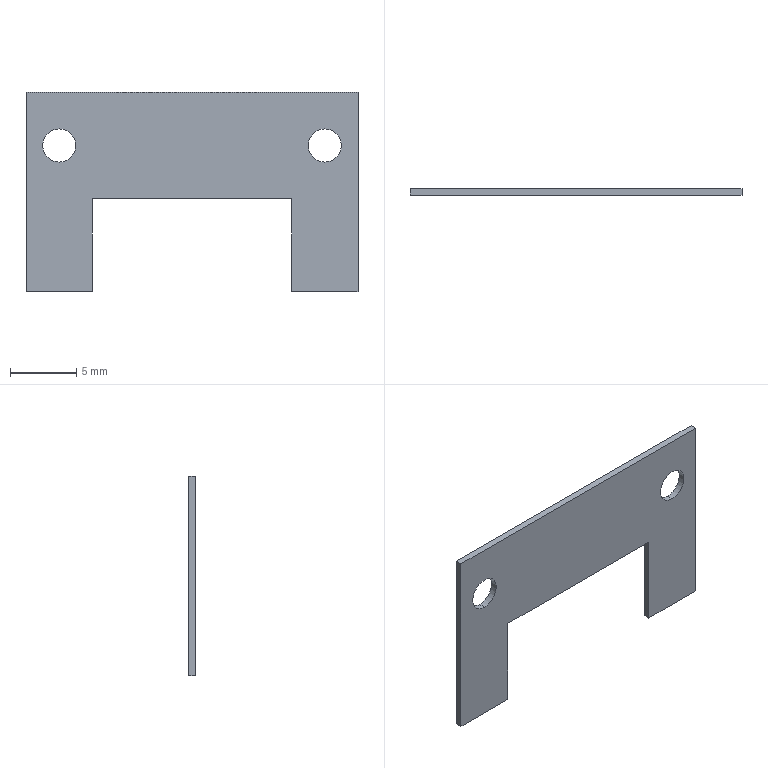Part | SolidWorks | features Extrusion 1 | 1 solid | 14 faces | box 25 x 0.5 x 15 mm | volume 130.091 mm3 | plane 10 | cylinder 4 | commonest cylinder face diameters 2.5 x4
STEP:
#1=CARTESIAN_POINT('',(-10.,0.5,-5.25));
#2=VERTEX_POINT('',#1);
#3=CARTESIAN_POINT('',(-10.,0.5,-2.75));
#4=VERTEX_POINT('',#3);
#5=CARTESIAN_POINT('',(-10.,0.5,-4.));
#6=DIRECTION('',(0.,1.,0.));
#7=DIRECTION('',(0.,0.,1.));
#8=AXIS2_PLACEMENT_3D('',#5,#6,#7);
#9=CIRCLE('',#8,1.25);
#10=EDGE_CURVE('',#2,#4,#9,.T.);
#11=ORIENTED_EDGE('',*,*,#10,.T.);
#12=CARTESIAN_POINT('',(-10.,0.,-2.75));
#13=VERTEX_POINT('',#12);
#14=CARTESIAN_POINT('',(-10.,0.5,-2.75));
#15=DIRECTION('',(0.,-1.,0.));
#16=VECTOR('',#15,1000.);
#17=LINE('',#14,#16);
#18=EDGE_CURVE('',#4,#13,#17,.T.);
#19=ORIENTED_EDGE('',*,*,#18,.T.);
#20=CARTESIAN_POINT('',(-10.,0.,-5.25));
#21=VERTEX_POINT('',#20);
#22=CARTESIAN_POINT('',(-10.,0.,-4.));
#23=DIRECTION('',(0.,1.,0.));
#24=DIRECTION('',(0.,0.,1.));
#25=AXIS2_PLACEMENT_3D('',#22,#23,#24);
#26=CIRCLE('',#25,1.25);
#27=EDGE_CURVE('',#21,#13,#26,.T.);
#28=ORIENTED_EDGE('',*,*,#27,.F.);
#29=CARTESIAN_POINT('',(-10.,0.5,-5.25));
#30=DIRECTION('',(0.,-1.,0.));
#31=VECTOR('',#30,1000.);
#32=LINE('',#29,#31);
#33=EDGE_CURVE('',#2,#21,#32,.T.);
#34=ORIENTED_EDGE('',*,*,#33,.F.);
#35=EDGE_LOOP('',(#11,#19,#28,#34));
#36=FACE_OUTER_BOUND('',#35,.T.);
#37=CARTESIAN_POINT('',(-10.,0.5,-4.));
#38=DIRECTION('',(0.,-1.,0.));
#39=DIRECTION('',(0.,0.,-1.));
#40=AXIS2_PLACEMENT_3D('',#37,#38,#39);
#41=CYLINDRICAL_SURFACE('',#40,1.25);
#42=ADVANCED_FACE('',(#36),#41,.F.);
#43=CARTESIAN_POINT('',(10.,0.5,-5.25));
#44=VERTEX_POINT('',#43);
#45=CARTESIAN_POINT('',(10.,0.5,-2.75));
#46=VERTEX_POINT('',#45);
#47=CARTESIAN_POINT('',(10.,0.5,-4.));
#48=DIRECTION('',(0.,1.,0.));
#49=DIRECTION('',(0.,0.,1.));
#50=AXIS2_PLACEMENT_3D('',#47,#48,#49);
#51=CIRCLE('',#50,1.25);
#52=EDGE_CURVE('',#44,#46,#51,.T.);
#53=ORIENTED_EDGE('',*,*,#52,.T.);
#54=CARTESIAN_POINT('',(10.,0.,-2.75));
#55=VERTEX_POINT('',#54);
#56=CARTESIAN_POINT('',(10.,0.5,-2.75));
#57=DIRECTION('',(0.,-1.,0.));
#58=VECTOR('',#57,1000.);
#59=LINE('',#56,#58);
#60=EDGE_CURVE('',#46,#55,#59,.T.);
#61=ORIENTED_EDGE('',*,*,#60,.T.);
#62=CARTESIAN_POINT('',(10.,0.,-5.25));
#63=VERTEX_POINT('',#62);
#64=CARTESIAN_POINT('',(10.,0.,-4.));
#65=DIRECTION('',(0.,1.,0.));
#66=DIRECTION('',(0.,0.,1.));
#67=AXIS2_PLACEMENT_3D('',#64,#65,#66);
#68=CIRCLE('',#67,1.25);
#69=EDGE_CURVE('',#63,#55,#68,.T.);
#70=ORIENTED_EDGE('',*,*,#69,.F.);
#71=CARTESIAN_POINT('',(10.,0.5,-5.25));
#72=DIRECTION('',(0.,-1.,0.));
#73=VECTOR('',#72,1000.);
#74=LINE('',#71,#73);
#75=EDGE_CURVE('',#44,#63,#74,.T.);
#76=ORIENTED_EDGE('',*,*,#75,.F.);
#77=EDGE_LOOP('',(#53,#61,#70,#76));
#78=FACE_OUTER_BOUND('',#77,.T.);
#79=CARTESIAN_POINT('',(10.,0.5,-4.));
#80=DIRECTION('',(0.,-1.,0.));
#81=DIRECTION('',(0.,0.,-1.));
#82=AXIS2_PLACEMENT_3D('',#79,#80,#81);
#83=CYLINDRICAL_SURFACE('',#82,1.25);
#84=ADVANCED_FACE('',(#78),#83,.F.);
#85=ORIENTED_EDGE('',*,*,#52,.F.);
#86=CARTESIAN_POINT('',(10.,0.5,-4.));
#87=DIRECTION('',(0.,1.,0.));
#88=DIRECTION('',(0.,0.,1.));
#89=AXIS2_PLACEMENT_3D('',#86,#87,#88);
#90=CIRCLE('',#89,1.25);
#91=EDGE_CURVE('',#46,#44,#90,.T.);
#92=ORIENTED_EDGE('',*,*,#91,.F.);
#93=EDGE_LOOP('',(#85,#92));
#94=FACE_BOUND('',#93,.T.);
#95=CARTESIAN_POINT('',(-12.5,0.5,-15.));
#96=VERTEX_POINT('',#95);
#97=CARTESIAN_POINT('',(-12.5,0.5,0.));
#98=VERTEX_POINT('',#97);
#99=CARTESIAN_POINT('',(-12.5,0.5,0.));
#100=DIRECTION('',(0.,0.,1.));
#101=VECTOR('',#100,1000.);
#102=LINE('',#99,#101);
#103=EDGE_CURVE('',#96,#98,#102,.T.);
#104=ORIENTED_EDGE('',*,*,#103,.T.);
#105=CARTESIAN_POINT('',(12.5,0.5,0.));
#106=VERTEX_POINT('',#105);
#107=CARTESIAN_POINT('',(-12.5,0.5,0.));
#108=DIRECTION('',(1.,0.,0.));
#109=VECTOR('',#108,1000.);
#110=LINE('',#107,#109);
#111=EDGE_CURVE('',#98,#106,#110,.T.);
#112=ORIENTED_EDGE('',*,*,#111,.T.);
#113=CARTESIAN_POINT('',(12.5,0.5,-15.));
#114=VERTEX_POINT('',#113);
#115=CARTESIAN_POINT('',(12.5,0.5,0.));
#116=DIRECTION('',(0.,0.,-1.));
#117=VECTOR('',#116,1000.);
#118=LINE('',#115,#117);
#119=EDGE_CURVE('',#106,#114,#118,.T.);
#120=ORIENTED_EDGE('',*,*,#119,.T.);
#121=CARTESIAN_POINT('',(7.5,0.5,-15.));
#122=VERTEX_POINT('',#121);
#123=CARTESIAN_POINT('',(12.5,0.5,-15.));
#124=DIRECTION('',(-1.,0.,0.));
#125=VECTOR('',#124,1000.);
#126=LINE('',#123,#125);
#127=EDGE_CURVE('',#114,#122,#126,.T.);
#128=ORIENTED_EDGE('',*,*,#127,.T.);
#129=CARTESIAN_POINT('',(7.5,0.5,-8.));
#130=VERTEX_POINT('',#129);
#131=CARTESIAN_POINT('',(7.5,0.5,-15.));
#132=DIRECTION('',(0.,0.,1.));
#133=VECTOR('',#132,1000.);
#134=LINE('',#131,#133);
#135=EDGE_CURVE('',#122,#130,#134,.T.);
#136=ORIENTED_EDGE('',*,*,#135,.T.);
#137=CARTESIAN_POINT('',(-7.5,0.5,-8.));
#138=VERTEX_POINT('',#137);
#139=CARTESIAN_POINT('',(7.5,0.5,-8.));
#140=DIRECTION('',(-1.,0.,0.));
#141=VECTOR('',#140,1000.);
#142=LINE('',#139,#141);
#143=EDGE_CURVE('',#130,#138,#142,.T.);
#144=ORIENTED_EDGE('',*,*,#143,.T.);
#145=CARTESIAN_POINT('',(-7.5,0.5,-15.));
#146=VERTEX_POINT('',#145);
#147=CARTESIAN_POINT('',(-7.5,0.5,-15.));
#148=DIRECTION('',(0.,0.,-1.));
#149=VECTOR('',#148,1000.);
#150=LINE('',#147,#149);
#151=EDGE_CURVE('',#138,#146,#150,.T.);
#152=ORIENTED_EDGE('',*,*,#151,.T.);
#153=CARTESIAN_POINT('',(-12.5,0.5,-15.));
#154=DIRECTION('',(-1.,0.,0.));
#155=VECTOR('',#154,1000.);
#156=LINE('',#153,#155);
#157=EDGE_CURVE('',#146,#96,#156,.T.);
#158=ORIENTED_EDGE('',*,*,#157,.T.);
#159=EDGE_LOOP('',(#104,#112,#120,#128,#136,#144,#152,#158));
#160=FACE_OUTER_BOUND('',#159,.T.);
#161=ORIENTED_EDGE('',*,*,#10,.F.);
#162=CARTESIAN_POINT('',(-10.,0.5,-4.));
#163=DIRECTION('',(0.,1.,0.));
#164=DIRECTION('',(0.,0.,1.));
#165=AXIS2_PLACEMENT_3D('',#162,#163,#164);
#166=CIRCLE('',#165,1.25);
#167=EDGE_CURVE('',#4,#2,#166,.T.);
#168=ORIENTED_EDGE('',*,*,#167,.F.);
#169=EDGE_LOOP('',(#161,#168));
#170=FACE_BOUND('',#169,.T.);
#171=CARTESIAN_POINT('',(-12.5,0.5,-15.));
#172=DIRECTION('',(0.,-1.,0.));
#173=DIRECTION('',(0.,0.,-1.));
#174=AXIS2_PLACEMENT_3D('',#171,#172,#173);
#175=PLANE('',#174);
#176=ADVANCED_FACE('',(#94,#160,#170),#175,.F.);
#177=ORIENTED_EDGE('',*,*,#69,.T.);
#178=CARTESIAN_POINT('',(10.,0.,-4.));
#179=DIRECTION('',(0.,1.,0.));
#180=DIRECTION('',(0.,0.,1.));
#181=AXIS2_PLACEMENT_3D('',#178,#179,#180);
#182=CIRCLE('',#181,1.25);
#183=EDGE_CURVE('',#55,#63,#182,.T.);
#184=ORIENTED_EDGE('',*,*,#183,.T.);
#185=EDGE_LOOP('',(#177,#184));
#186=FACE_BOUND('',#185,.T.);
#187=CARTESIAN_POINT('',(-12.5,0.,-15.));
#188=VERTEX_POINT('',#187);
#189=CARTESIAN_POINT('',(-12.5,0.,0.));
#190=VERTEX_POINT('',#189);
#191=CARTESIAN_POINT('',(-12.5,0.,0.));
#192=DIRECTION('',(0.,0.,1.));
#193=VECTOR('',#192,1000.);
#194=LINE('',#191,#193);
#195=EDGE_CURVE('',#188,#190,#194,.T.);
#196=ORIENTED_EDGE('',*,*,#195,.F.);
#197=CARTESIAN_POINT('',(-7.5,0.,-15.));
#198=VERTEX_POINT('',#197);
#199=CARTESIAN_POINT('',(-12.5,0.,-15.));
#200=DIRECTION('',(-1.,0.,0.));
#201=VECTOR('',#200,1000.);
#202=LINE('',#199,#201);
#203=EDGE_CURVE('',#198,#188,#202,.T.);
#204=ORIENTED_EDGE('',*,*,#203,.F.);
#205=CARTESIAN_POINT('',(-7.5,0.,-8.));
#206=VERTEX_POINT('',#205);
#207=CARTESIAN_POINT('',(-7.5,0.,-15.));
#208=DIRECTION('',(0.,0.,-1.));
#209=VECTOR('',#208,1000.);
#210=LINE('',#207,#209);
#211=EDGE_CURVE('',#206,#198,#210,.T.);
#212=ORIENTED_EDGE('',*,*,#211,.F.);
#213=CARTESIAN_POINT('',(7.5,0.,-8.));
#214=VERTEX_POINT('',#213);
#215=CARTESIAN_POINT('',(7.5,0.,-8.));
#216=DIRECTION('',(-1.,0.,0.));
#217=VECTOR('',#216,1000.);
#218=LINE('',#215,#217);
#219=EDGE_CURVE('',#214,#206,#218,.T.);
#220=ORIENTED_EDGE('',*,*,#219,.F.);
#221=CARTESIAN_POINT('',(7.5,0.,-15.));
#222=VERTEX_POINT('',#221);
#223=CARTESIAN_POINT('',(7.5,0.,-15.));
#224=DIRECTION('',(0.,0.,1.));
#225=VECTOR('',#224,1000.);
#226=LINE('',#223,#225);
#227=EDGE_CURVE('',#222,#214,#226,.T.);
#228=ORIENTED_EDGE('',*,*,#227,.F.);
#229=CARTESIAN_POINT('',(12.5,0.,-15.));
#230=VERTEX_POINT('',#229);
#231=CARTESIAN_POINT('',(12.5,0.,-15.));
#232=DIRECTION('',(-1.,0.,0.));
#233=VECTOR('',#232,1000.);
#234=LINE('',#231,#233);
#235=EDGE_CURVE('',#230,#222,#234,.T.);
#236=ORIENTED_EDGE('',*,*,#235,.F.);
#237=CARTESIAN_POINT('',(12.5,0.,0.));
#238=VERTEX_POINT('',#237);
#239=CARTESIAN_POINT('',(12.5,0.,0.));
#240=DIRECTION('',(0.,0.,-1.));
#241=VECTOR('',#240,1000.);
#242=LINE('',#239,#241);
#243=EDGE_CURVE('',#238,#230,#242,.T.);
#244=ORIENTED_EDGE('',*,*,#243,.F.);
#245=CARTESIAN_POINT('',(-12.5,0.,0.));
#246=DIRECTION('',(1.,0.,0.));
#247=VECTOR('',#246,1000.);
#248=LINE('',#245,#247);
#249=EDGE_CURVE('',#190,#238,#248,.T.);
#250=ORIENTED_EDGE('',*,*,#249,.F.);
#251=EDGE_LOOP('',(#196,#204,#212,#220,#228,#236,#244,#250));
#252=FACE_OUTER_BOUND('',#251,.T.);
#253=ORIENTED_EDGE('',*,*,#27,.T.);
#254=CARTESIAN_POINT('',(-10.,0.,-4.));
#255=DIRECTION('',(0.,1.,0.));
#256=DIRECTION('',(0.,0.,1.));
#257=AXIS2_PLACEMENT_3D('',#254,#255,#256);
#258=CIRCLE('',#257,1.25);
#259=EDGE_CURVE('',#13,#21,#258,.T.);
#260=ORIENTED_EDGE('',*,*,#259,.T.);
#261=EDGE_LOOP('',(#253,#260));
#262=FACE_BOUND('',#261,.T.);
#263=CARTESIAN_POINT('',(-12.5,0.,-15.));
#264=DIRECTION('',(0.,-1.,0.));
#265=DIRECTION('',(0.,0.,-1.));
#266=AXIS2_PLACEMENT_3D('',#263,#264,#265);
#267=PLANE('',#266);
#268=ADVANCED_FACE('',(#186,#252,#262),#267,.T.);
#269=ORIENTED_EDGE('',*,*,#195,.T.);
#270=CARTESIAN_POINT('',(-12.5,0.5,0.));
#271=DIRECTION('',(0.,-1.,0.));
#272=VECTOR('',#271,1000.);
#273=LINE('',#270,#272);
#274=EDGE_CURVE('',#98,#190,#273,.T.);
#275=ORIENTED_EDGE('',*,*,#274,.F.);
#276=ORIENTED_EDGE('',*,*,#103,.F.);
#277=CARTESIAN_POINT('',(-12.5,0.5,-15.));
#278=DIRECTION('',(0.,-1.,0.));
#279=VECTOR('',#278,1000.);
#280=LINE('',#277,#279);
#281=EDGE_CURVE('',#96,#188,#280,.T.);
#282=ORIENTED_EDGE('',*,*,#281,.T.);
#283=EDGE_LOOP('',(#269,#275,#276,#282));
#284=FACE_OUTER_BOUND('',#283,.T.);
#285=CARTESIAN_POINT('',(-12.5,0.5,0.));
#286=DIRECTION('',(1.,0.,0.));
#287=DIRECTION('',(0.,0.,-1.));
#288=AXIS2_PLACEMENT_3D('',#285,#286,#287);
#289=PLANE('',#288);
#290=ADVANCED_FACE('',(#284),#289,.F.);
#291=ORIENTED_EDGE('',*,*,#249,.T.);
#292=CARTESIAN_POINT('',(12.5,0.5,0.));
#293=DIRECTION('',(0.,-1.,0.));
#294=VECTOR('',#293,1000.);
#295=LINE('',#292,#294);
#296=EDGE_CURVE('',#106,#238,#295,.T.);
#297=ORIENTED_EDGE('',*,*,#296,.F.);
#298=ORIENTED_EDGE('',*,*,#111,.F.);
#299=ORIENTED_EDGE('',*,*,#274,.T.);
#300=EDGE_LOOP('',(#291,#297,#298,#299));
#301=FACE_OUTER_BOUND('',#300,.T.);
#302=CARTESIAN_POINT('',(-12.5,0.5,0.));
#303=DIRECTION('',(0.,0.,-1.));
#304=DIRECTION('',(-1.,0.,0.));
#305=AXIS2_PLACEMENT_3D('',#302,#303,#304);
#306=PLANE('',#305);
#307=ADVANCED_FACE('',(#301),#306,.F.);
#308=ORIENTED_EDGE('',*,*,#243,.T.);
#309=CARTESIAN_POINT('',(12.5,0.5,-15.));
#310=DIRECTION('',(0.,-1.,0.));
#311=VECTOR('',#310,1000.);
#312=LINE('',#309,#311);
#313=EDGE_CURVE('',#114,#230,#312,.T.);
#314=ORIENTED_EDGE('',*,*,#313,.F.);
#315=ORIENTED_EDGE('',*,*,#119,.F.);
#316=ORIENTED_EDGE('',*,*,#296,.T.);
#317=EDGE_LOOP('',(#308,#314,#315,#316));
#318=FACE_OUTER_BOUND('',#317,.T.);
#319=CARTESIAN_POINT('',(12.5,0.5,0.));
#320=DIRECTION('',(-1.,0.,0.));
#321=DIRECTION('',(0.,0.,1.));
#322=AXIS2_PLACEMENT_3D('',#319,#320,#321);
#323=PLANE('',#322);
#324=ADVANCED_FACE('',(#318),#323,.F.);
#325=ORIENTED_EDGE('',*,*,#235,.T.);
#326=CARTESIAN_POINT('',(7.5,0.5,-15.));
#327=DIRECTION('',(0.,-1.,0.));
#328=VECTOR('',#327,1000.);
#329=LINE('',#326,#328);
#330=EDGE_CURVE('',#122,#222,#329,.T.);
#331=ORIENTED_EDGE('',*,*,#330,.F.);
#332=ORIENTED_EDGE('',*,*,#127,.F.);
#333=ORIENTED_EDGE('',*,*,#313,.T.);
#334=EDGE_LOOP('',(#325,#331,#332,#333));
#335=FACE_OUTER_BOUND('',#334,.T.);
#336=CARTESIAN_POINT('',(12.5,0.5,-15.));
#337=DIRECTION('',(0.,0.,1.));
#338=DIRECTION('',(1.,0.,0.));
#339=AXIS2_PLACEMENT_3D('',#336,#337,#338);
#340=PLANE('',#339);
#341=ADVANCED_FACE('',(#335),#340,.F.);
#342=ORIENTED_EDGE('',*,*,#227,.T.);
#343=CARTESIAN_POINT('',(7.5,0.5,-8.));
#344=DIRECTION('',(0.,-1.,0.));
#345=VECTOR('',#344,1000.);
#346=LINE('',#343,#345);
#347=EDGE_CURVE('',#130,#214,#346,.T.);
#348=ORIENTED_EDGE('',*,*,#347,.F.);
#349=ORIENTED_EDGE('',*,*,#135,.F.);
#350=ORIENTED_EDGE('',*,*,#330,.T.);
#351=EDGE_LOOP('',(#342,#348,#349,#350));
#352=FACE_OUTER_BOUND('',#351,.T.);
#353=CARTESIAN_POINT('',(7.5,0.5,-15.));
#354=DIRECTION('',(1.,0.,0.));
#355=DIRECTION('',(0.,0.,-1.));
#356=AXIS2_PLACEMENT_3D('',#353,#354,#355);
#357=PLANE('',#356);
#358=ADVANCED_FACE('',(#352),#357,.F.);
#359=ORIENTED_EDGE('',*,*,#219,.T.);
#360=CARTESIAN_POINT('',(-7.5,0.5,-8.));
#361=DIRECTION('',(0.,-1.,0.));
#362=VECTOR('',#361,1000.);
#363=LINE('',#360,#362);
#364=EDGE_CURVE('',#138,#206,#363,.T.);
#365=ORIENTED_EDGE('',*,*,#364,.F.);
#366=ORIENTED_EDGE('',*,*,#143,.F.);
#367=ORIENTED_EDGE('',*,*,#347,.T.);
#368=EDGE_LOOP('',(#359,#365,#366,#367));
#369=FACE_OUTER_BOUND('',#368,.T.);
#370=CARTESIAN_POINT('',(7.5,0.5,-8.));
#371=DIRECTION('',(0.,0.,1.));
#372=DIRECTION('',(1.,0.,0.));
#373=AXIS2_PLACEMENT_3D('',#370,#371,#372);
#374=PLANE('',#373);
#375=ADVANCED_FACE('',(#369),#374,.F.);
#376=ORIENTED_EDGE('',*,*,#211,.T.);
#377=CARTESIAN_POINT('',(-7.5,0.5,-15.));
#378=DIRECTION('',(0.,-1.,0.));
#379=VECTOR('',#378,1000.);
#380=LINE('',#377,#379);
#381=EDGE_CURVE('',#146,#198,#380,.T.);
#382=ORIENTED_EDGE('',*,*,#381,.F.);
#383=ORIENTED_EDGE('',*,*,#151,.F.);
#384=ORIENTED_EDGE('',*,*,#364,.T.);
#385=EDGE_LOOP('',(#376,#382,#383,#384));
#386=FACE_OUTER_BOUND('',#385,.T.);
#387=CARTESIAN_POINT('',(-7.5,0.5,-15.));
#388=DIRECTION('',(-1.,0.,0.));
#389=DIRECTION('',(0.,0.,1.));
#390=AXIS2_PLACEMENT_3D('',#387,#388,#389);
#391=PLANE('',#390);
#392=ADVANCED_FACE('',(#386),#391,.F.);
#393=ORIENTED_EDGE('',*,*,#203,.T.);
#394=ORIENTED_EDGE('',*,*,#281,.F.);
#395=ORIENTED_EDGE('',*,*,#157,.F.);
#396=ORIENTED_EDGE('',*,*,#381,.T.);
#397=EDGE_LOOP('',(#393,#394,#395,#396));
#398=FACE_OUTER_BOUND('',#397,.T.);
#399=CARTESIAN_POINT('',(-12.5,0.5,-15.));
#400=DIRECTION('',(0.,0.,1.));
#401=DIRECTION('',(1.,0.,0.));
#402=AXIS2_PLACEMENT_3D('',#399,#400,#401);
#403=PLANE('',#402);
#404=ADVANCED_FACE('',(#398),#403,.F.);
#405=ORIENTED_EDGE('',*,*,#60,.F.);
#406=ORIENTED_EDGE('',*,*,#91,.T.);
#407=ORIENTED_EDGE('',*,*,#75,.T.);
#408=ORIENTED_EDGE('',*,*,#183,.F.);
#409=EDGE_LOOP('',(#405,#406,#407,#408));
#410=FACE_OUTER_BOUND('',#409,.T.);
#411=CARTESIAN_POINT('',(10.,0.5,-4.));
#412=DIRECTION('',(0.,-1.,0.));
#413=DIRECTION('',(0.,0.,-1.));
#414=AXIS2_PLACEMENT_3D('',#411,#412,#413);
#415=CYLINDRICAL_SURFACE('',#414,1.25);
#416=ADVANCED_FACE('',(#410),#415,.F.);
#417=ORIENTED_EDGE('',*,*,#18,.F.);
#418=ORIENTED_EDGE('',*,*,#167,.T.);
#419=ORIENTED_EDGE('',*,*,#33,.T.);
#420=ORIENTED_EDGE('',*,*,#259,.F.);
#421=EDGE_LOOP('',(#417,#418,#419,#420));
#422=FACE_OUTER_BOUND('',#421,.T.);
#423=CARTESIAN_POINT('',(-10.,0.5,-4.));
#424=DIRECTION('',(0.,-1.,0.));
#425=DIRECTION('',(0.,0.,-1.));
#426=AXIS2_PLACEMENT_3D('',#423,#424,#425);
#427=CYLINDRICAL_SURFACE('',#426,1.25);
#428=ADVANCED_FACE('',(#422),#427,.F.);
#429=CLOSED_SHELL('',(#42,#84,#176,#268,#290,#307,#324,#341,#358,#375,#392,#404,#416,#428));
#430=MANIFOLD_SOLID_BREP('',#429);
#431=CARTESIAN_POINT('',(0.,0.,0.));
#432=DIRECTION('',(0.,0.,1.));
#433=DIRECTION('',(1.,0.,0.));
#434=AXIS2_PLACEMENT_3D('',#431,#432,#433);
#435=(LENGTH_UNIT()NAMED_UNIT(*)SI_UNIT(.MILLI.,.METRE.));
#436=UNCERTAINTY_MEASURE_WITH_UNIT(LENGTH_MEASURE(0.00001),#435,'','');
#437=(NAMED_UNIT(*)PLANE_ANGLE_UNIT()SI_UNIT($,.RADIAN.));
#438=(NAMED_UNIT(*)SI_UNIT($,.STERADIAN.)SOLID_ANGLE_UNIT());
#439=(GEOMETRIC_REPRESENTATION_CONTEXT(3)GLOBAL_UNCERTAINTY_ASSIGNED_CONTEXT((#436))GLOBAL_UNIT_ASSIGNED_CONTEXT((#435,#437,#438))REPRESENTATION_CONTEXT('',''));
#440=ADVANCED_BREP_SHAPE_REPRESENTATION('',(#430,#434),#439);